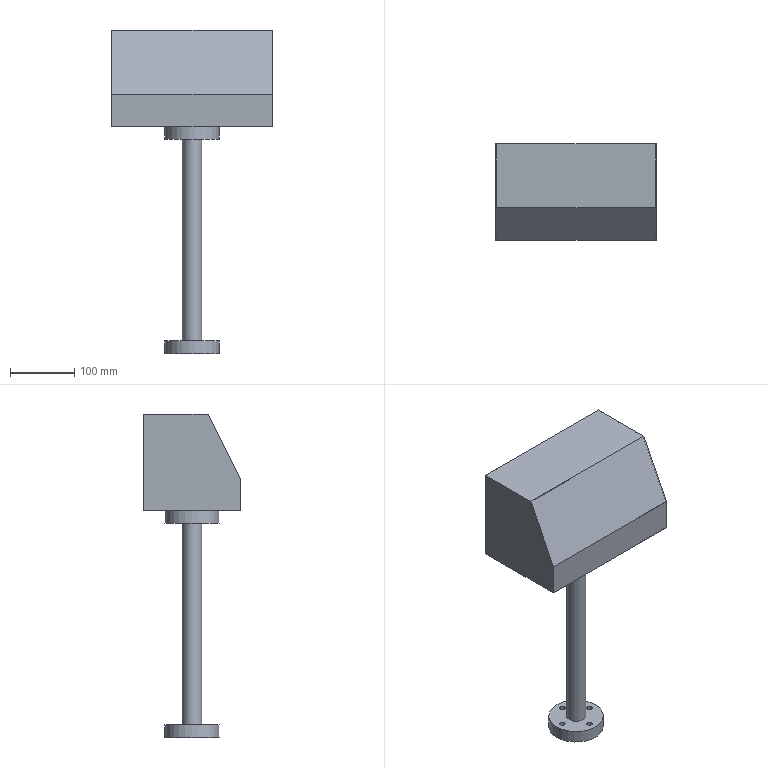Part | STEP file | Touch screen assembly | 5 solids | 44 faces | box 250 x 150 x 505 mm | volume 675168 mm3 | plane 25 | cylinder 19 | commonest cylinder face diameters 5.5 x4 8.5 x4 30 x3 35.5 x3 10.7 x2 85 x2